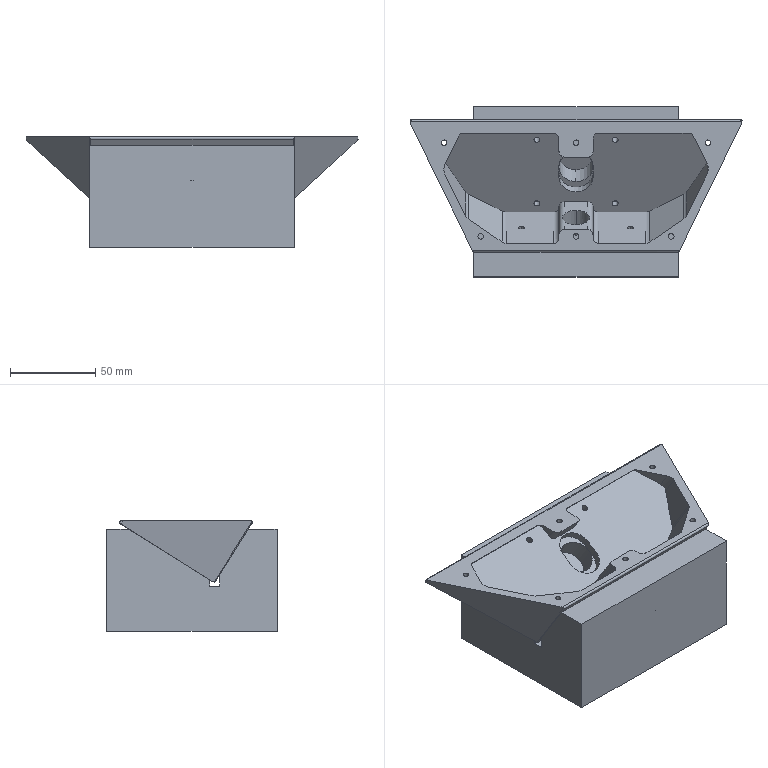Part | 2 solids | 97 faces | box 195.124 x 100 x 65 mm | volume 670273 mm3 | cylinder 54 | plane 43 | commonest cylinder face diameters 3.3 x16 6 x10 3.5 x8 2 x6 10 x6 20 x4